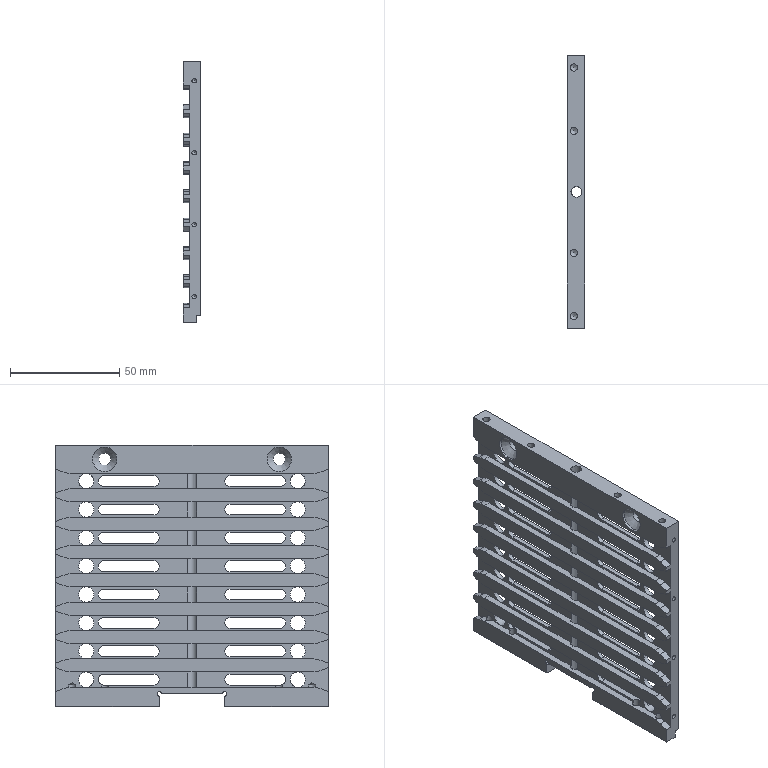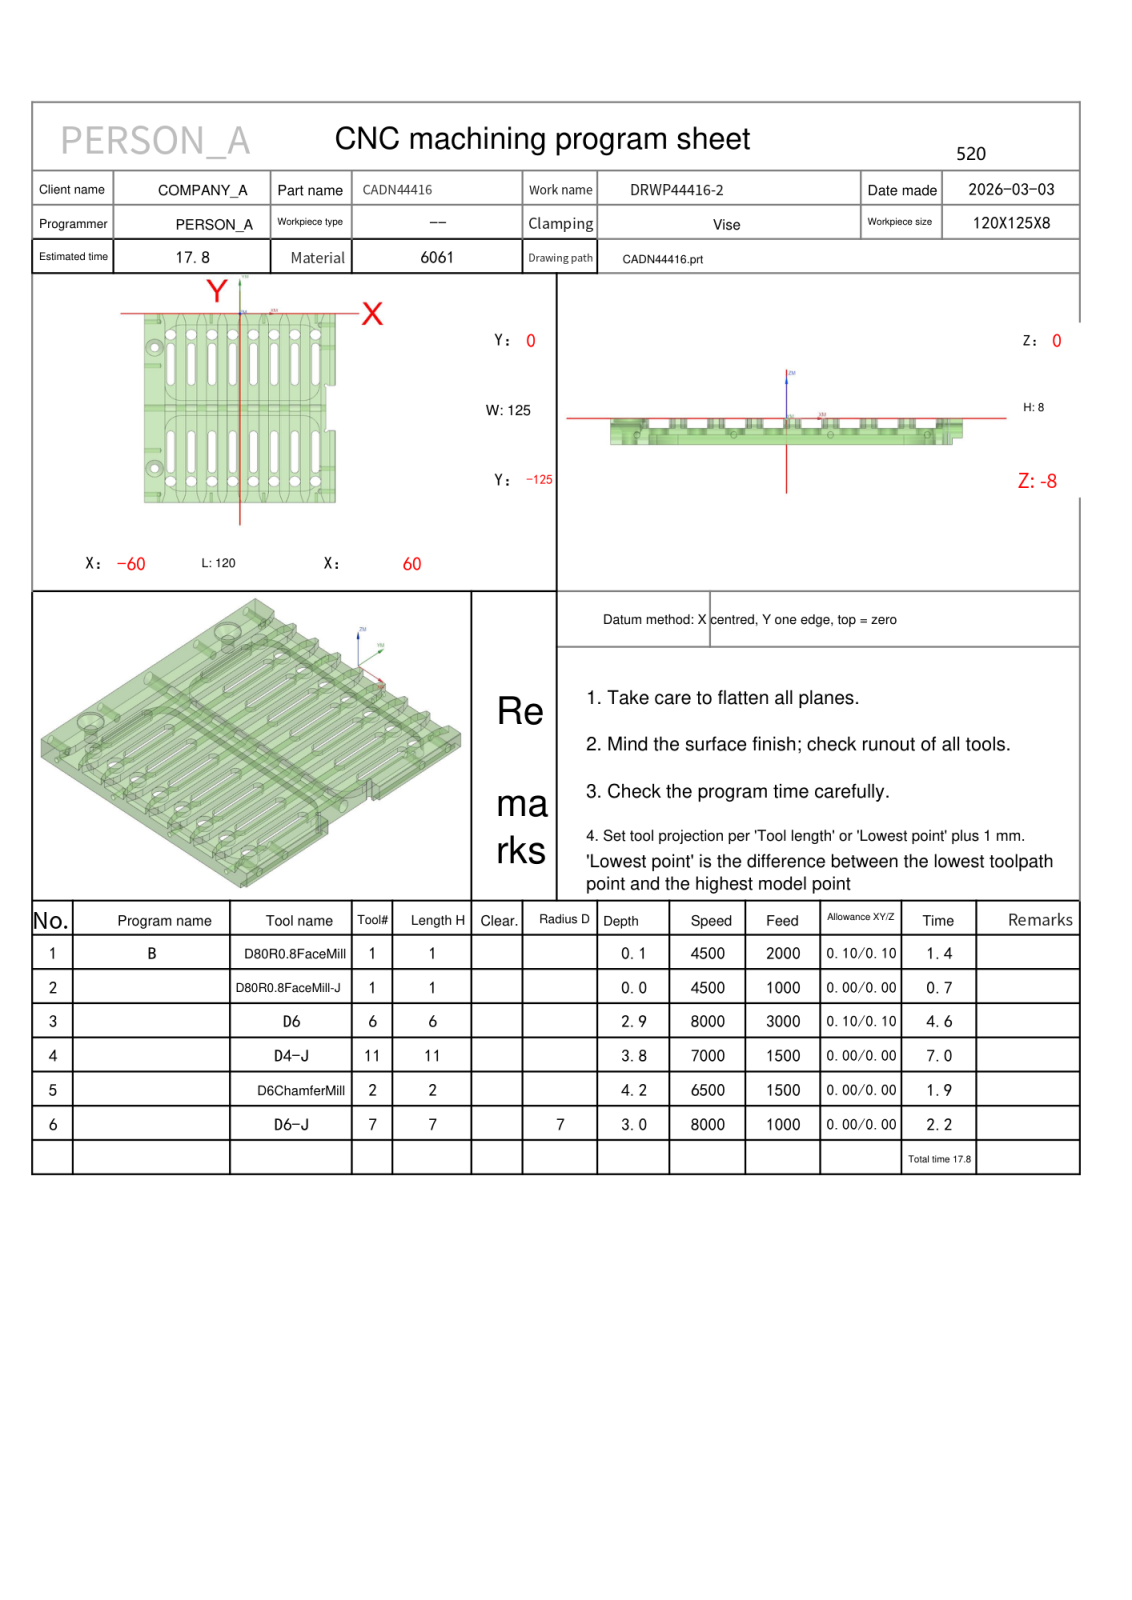NC program | NX | posted by the shop | part box 8 x 125 x 120 mm
Lines 1 to 1103 of 79132:
%
O0001
(Machine time: 19.00 MIN)
(===Total Tool:5===)
(T1=D80R0.8 FaceMill D=80.  R=0.8  D-  H01 Z=-0.   )
(T6=D6      D=6.   R=0.   D-  H06 Z=-2.9  )
(T11=D4-J   D=4.   R=0.   D-  H11 Z=-3.85 )
(T2=D6ChamferMill   D=6.   R=0.   D-  H02 Z=-4.2  )
(T7=D6-J    D=6.   R=0.   D7  H07 Z=-3.   )
G80 G90 G17 G49 G40
G91 G28 Z0
M01
N1 T01 M06
(D80R0.8 FaceMill  D=80. R=0.8 H=01 ce=0.10 di=0.10)
G00 G90 G54 X-112.097 Y-23.903 M03 S4500
G43 H01 Z50.
M08
Z3.525
G01 Z1.525 F2000.
X-100.097
X92.1
G02 X100.097 Y-31.9 I-.003 J-8.
G01 Y-37.403
Y-50.822
G02 X92.099 Y-58.82 I-8. J.002
G01 X-92.897
G03 X-100.097 Y-66.02 I0.0 J-7.2
G01 Y-85.737
G03 X-92.097 Y-93.737 I8. J0.0
G01 X100.097
X112.097
Z3.525
G00 X-112.097 Y-23.903
Z3.05
G01 Z1.05
X-100.097
X92.1
G02 X100.097 Y-31.9 I-.003 J-8.
G01 Y-37.403
Y-50.822
G02 X92.099 Y-58.82 I-8. J.002
G01 X-92.897
G03 X-100.097 Y-66.02 I0.0 J-7.2
G01 Y-85.737
G03 X-92.097 Y-93.737 I8. J0.0
G01 X100.097
X112.097
Z3.05
G00 X-112.097 Y-23.903
Z2.575
G01 Z.575
X-100.097
X92.1
G02 X100.097 Y-31.9 I-.003 J-8.
G01 Y-37.403
Y-50.822
G02 X92.099 Y-58.82 I-8. J.002
G01 X-92.897
G03 X-100.097 Y-66.02 I0.0 J-7.2
G01 Y-85.737
G03 X-92.097 Y-93.737 I8. J0.0
G01 X100.097
X112.097
Z2.575
G00 X-112.097 Y-23.903
Z2.1
G01 Z.1
X-100.097
X92.1
G02 X100.097 Y-31.9 I-.003 J-8.
G01 Y-37.403
Y-50.822
G02 X92.099 Y-58.82 I-8. J.002
G01 X-92.897
G03 X-100.097 Y-66.02 I0.0 J-7.2
G01 Y-85.737
G03 X-92.097 Y-93.737 I8. J0.0
G01 X100.097
X112.097
Z2.1
G00 Z50.
G91 G28 Z0.0
M05
M09
G91 G28 Z0.0
M01
N2 T01 M06
(D80R0.8 FaceMill-J  D=80. R=0.8 H=01 ce=0.00 di=0.00)
G00 G90 G54 X-111.999 Y-24.001 M03 S4500
G43 H01 Z50.
M08
Z2.
G01 Z0.0 F1000.
X-99.999
X92.002
G02 X99.999 Y-31.998 I-.003 J-8.
G01 Y-37.501
Y-50.823
G02 X92.002 Y-58.82 I-8. J.003
G01 X-92.799
G03 X-99.999 Y-66.02 I0.0 J-7.2
G01 Y-85.639
G03 X-91.999 Y-93.639 I8. J0.0
G01 X99.999
X111.999
Z2.
G00 Z50.
G91 G28 Z0.0
M05
M09
G91 G28 Z0.0
M01
N3 T06 M06
(D6  D=6. R=0. H=06 ce=0.10 di=0.10)
G00 G90 G54 X-43.5 Y-131. M03 S8000
G43 H06 Z11.805
M08
Z1.017
G01 Z-.483 F3000.
Y-127.94
X-46.773
X-44.69 Y-122.217
G03 X-43.9 Y-117.737 I-12.31 J4.48
G01 Y-7.263
G03 X-44.69 Y-2.783 I-13.1 J0.0
G01 X-46.773 Y2.94
X-40.227
X-42.31 Y-2.783
G03 X-43.1 Y-7.263 I12.31 J-4.48
G01 Y-117.737
G03 X-42.31 Y-122.217 I13.1 J0.0
G01 X-40.227 Y-127.94
X-43.5
X-44.
Y-131.
Z1.017
G00 X-43.5
Z.533
G01 Z-.967
Y-127.94
X-46.773
X-44.69 Y-122.217
G03 X-43.9 Y-117.737 I-12.31 J4.48
G01 Y-7.263
G03 X-44.69 Y-2.783 I-13.1 J0.0
G01 X-46.773 Y2.94
X-40.227
X-42.31 Y-2.783
G03 X-43.1 Y-7.263 I12.31 J-4.48
G01 Y-117.737
G03 X-42.31 Y-122.217 I13.1 J0.0
G01 X-40.227 Y-127.94
X-43.5
X-44.
Y-131.
Z.533
G00 X-43.5
Z.05
G01 Z-1.45
Y-127.94
X-46.773
X-44.69 Y-122.217
G03 X-43.9 Y-117.737 I-12.31 J4.48
G01 Y-7.263
G03 X-44.69 Y-2.783 I-13.1 J0.0
G01 X-46.773 Y2.94
X-40.227
X-42.31 Y-2.783
G03 X-43.1 Y-7.263 I12.31 J-4.48
G01 Y-117.737
G03 X-42.31 Y-122.217 I13.1 J0.0
G01 X-40.227 Y-127.94
X-43.5
X-44.
Y-131.
Z.05
G00 X-43.5
Z-.433
G01 Z-1.933
Y-127.94
X-46.773
X-44.69 Y-122.217
G03 X-43.9 Y-117.737 I-12.31 J4.48
G01 Y-7.263
G03 X-44.69 Y-2.783 I-13.1 J0.0
G01 X-46.773 Y2.94
X-40.227
X-42.31 Y-2.783
G03 X-43.1 Y-7.263 I12.31 J-4.48
G01 Y-117.737
G03 X-42.31 Y-122.217 I13.1 J0.0
G01 X-40.227 Y-127.94
X-43.5
X-44.
Y-131.
Z-.433
G00 X-43.5
Z-.917
G01 Z-2.417
Y-127.94
X-46.773
X-44.69 Y-122.217
G03 X-43.9 Y-117.737 I-12.31 J4.48
G01 Y-7.263
G03 X-44.69 Y-2.783 I-13.1 J0.0
G01 X-46.773 Y2.94
X-40.227
X-42.31 Y-2.783
G03 X-43.1 Y-7.263 I12.31 J-4.48
G01 Y-117.737
G03 X-42.31 Y-122.217 I13.1 J0.0
G01 X-40.227 Y-127.94
X-43.5
X-44.
Y-131.
Z-.917
G00 X-43.5
Z-1.4
G01 Z-2.9
Y-127.94
X-46.773
X-44.69 Y-122.217
G03 X-43.9 Y-117.737 I-12.31 J4.48
G01 Y-7.263
G03 X-44.69 Y-2.783 I-13.1 J0.0
G01 X-46.773 Y2.94
X-40.227
X-42.31 Y-2.783
G03 X-43.1 Y-7.263 I12.31 J-4.48
G01 Y-117.737
G03 X-42.31 Y-122.217 I13.1 J0.0
G01 X-40.227 Y-127.94
X-43.5
X-44.
Y-131.
Z-1.4
G00 Z3.
X-30.5
Z1.017
G01 Z-.483
Y-127.94
X-33.773
X-31.69 Y-122.217
G03 X-30.9 Y-117.737 I-12.31 J4.48
G01 Y-7.263
G03 X-31.69 Y-2.783 I-13.1 J0.0
G01 X-33.773 Y2.94
X-27.227
X-29.31 Y-2.783
G03 X-30.1 Y-7.263 I12.31 J-4.48
G01 Y-117.737
G03 X-29.31 Y-122.217 I13.1 J0.0
G01 X-27.227 Y-127.94
X-30.5
X-31.
Y-131.
Z1.017
G00 X-30.5
Z.533
G01 Z-.967
Y-127.94
X-33.773
X-31.69 Y-122.217
G03 X-30.9 Y-117.737 I-12.31 J4.48
G01 Y-7.263
G03 X-31.69 Y-2.783 I-13.1 J0.0
G01 X-33.773 Y2.94
X-27.227
X-29.31 Y-2.783
G03 X-30.1 Y-7.263 I12.31 J-4.48
G01 Y-117.737
G03 X-29.31 Y-122.217 I13.1 J0.0
G01 X-27.227 Y-127.94
X-30.5
X-31.
Y-131.
Z.533
G00 X-30.5
Z.05
G01 Z-1.45
Y-127.94
X-33.773
X-31.69 Y-122.217
G03 X-30.9 Y-117.737 I-12.31 J4.48
G01 Y-7.263
G03 X-31.69 Y-2.783 I-13.1 J0.0
G01 X-33.773 Y2.94
X-27.227
X-29.31 Y-2.783
G03 X-30.1 Y-7.263 I12.31 J-4.48
G01 Y-117.737
G03 X-29.31 Y-122.217 I13.1 J0.0
G01 X-27.227 Y-127.94
X-30.5
X-31.
Y-131.
Z.05
G00 X-30.5
Z-.433
G01 Z-1.933
Y-127.94
X-33.773
X-31.69 Y-122.217
G03 X-30.9 Y-117.737 I-12.31 J4.48
G01 Y-7.263
G03 X-31.69 Y-2.783 I-13.1 J0.0
G01 X-33.773 Y2.94
X-27.227
X-29.31 Y-2.783
G03 X-30.1 Y-7.263 I12.31 J-4.48
G01 Y-117.737
G03 X-29.31 Y-122.217 I13.1 J0.0
G01 X-27.227 Y-127.94
X-30.5
X-31.
Y-131.
Z-.433
G00 X-30.5
Z-.917
G01 Z-2.417
Y-127.94
X-33.773
X-31.69 Y-122.217
G03 X-30.9 Y-117.737 I-12.31 J4.48
G01 Y-7.263
G03 X-31.69 Y-2.783 I-13.1 J0.0
G01 X-33.773 Y2.94
X-27.227
X-29.31 Y-2.783
G03 X-30.1 Y-7.263 I12.31 J-4.48
G01 Y-117.737
G03 X-29.31 Y-122.217 I13.1 J0.0
G01 X-27.227 Y-127.94
X-30.5
X-31.
Y-131.
Z-.917
G00 X-30.5
Z-1.4
G01 Z-2.9
Y-127.94
X-33.773
X-31.69 Y-122.217
G03 X-30.9 Y-117.737 I-12.31 J4.48
G01 Y-7.263
G03 X-31.69 Y-2.783 I-13.1 J0.0
G01 X-33.773 Y2.94
X-27.227
X-29.31 Y-2.783
G03 X-30.1 Y-7.263 I12.31 J-4.48
G01 Y-117.737
G03 X-29.31 Y-122.217 I13.1 J0.0
G01 X-27.227 Y-127.94
X-30.5
X-31.
Y-131.
Z-1.4
G00 Z3.
X-17.5
Z1.017
G01 Z-.483
Y-127.94
X-20.773
X-18.69 Y-122.217
G03 X-17.9 Y-117.737 I-12.31 J4.48
G01 Y-7.263
G03 X-18.69 Y-2.783 I-13.1 J0.0
G01 X-20.773 Y2.94
X-14.227
X-16.31 Y-2.783
G03 X-17.1 Y-7.263 I12.31 J-4.48
G01 Y-117.737
G03 X-16.31 Y-122.217 I13.1 J0.0
G01 X-14.227 Y-127.94
X-17.5
X-18.
Y-131.
Z1.017
G00 X-17.5
Z.533
G01 Z-.967
Y-127.94
X-20.773
X-18.69 Y-122.217
G03 X-17.9 Y-117.737 I-12.31 J4.48
G01 Y-7.263
G03 X-18.69 Y-2.783 I-13.1 J0.0
G01 X-20.773 Y2.94
X-14.227
X-16.31 Y-2.783
G03 X-17.1 Y-7.263 I12.31 J-4.48
G01 Y-117.737
G03 X-16.31 Y-122.217 I13.1 J0.0
G01 X-14.227 Y-127.94
X-17.5
X-18.
Y-131.
Z.533
G00 X-17.5
Z.05
G01 Z-1.45
Y-127.94
X-20.773
X-18.69 Y-122.217
G03 X-17.9 Y-117.737 I-12.31 J4.48
G01 Y-7.263
G03 X-18.69 Y-2.783 I-13.1 J0.0
G01 X-20.773 Y2.94
X-14.227
X-16.31 Y-2.783
G03 X-17.1 Y-7.263 I12.31 J-4.48
G01 Y-117.737
G03 X-16.31 Y-122.217 I13.1 J0.0
G01 X-14.227 Y-127.94
X-17.5
X-18.
Y-131.
Z.05
G00 X-17.5
Z-.433
G01 Z-1.933
Y-127.94
X-20.773
X-18.69 Y-122.217
G03 X-17.9 Y-117.737 I-12.31 J4.48
G01 Y-7.263
G03 X-18.69 Y-2.783 I-13.1 J0.0
G01 X-20.773 Y2.94
X-14.227
X-16.31 Y-2.783
G03 X-17.1 Y-7.263 I12.31 J-4.48
G01 Y-117.737
G03 X-16.31 Y-122.217 I13.1 J0.0
G01 X-14.227 Y-127.94
X-17.5
X-18.
Y-131.
Z-.433
G00 X-17.5
Z-.917
G01 Z-2.417
Y-127.94
X-20.773
X-18.69 Y-122.217
G03 X-17.9 Y-117.737 I-12.31 J4.48
G01 Y-7.263
G03 X-18.69 Y-2.783 I-13.1 J0.0
G01 X-20.773 Y2.94
X-14.227
X-16.31 Y-2.783
G03 X-17.1 Y-7.263 I12.31 J-4.48
G01 Y-117.737
G03 X-16.31 Y-122.217 I13.1 J0.0
G01 X-14.227 Y-127.94
X-17.5
X-18.
Y-131.
Z-.917
G00 X-17.5
Z-1.4
G01 Z-2.9
Y-127.94
X-20.773
X-18.69 Y-122.217
G03 X-17.9 Y-117.737 I-12.31 J4.48
G01 Y-7.263
G03 X-18.69 Y-2.783 I-13.1 J0.0
G01 X-20.773 Y2.94
X-14.227
X-16.31 Y-2.783
G03 X-17.1 Y-7.263 I12.31 J-4.48
G01 Y-117.737
G03 X-16.31 Y-122.217 I13.1 J0.0
G01 X-14.227 Y-127.94
X-17.5
X-18.
Y-131.
Z-1.4
G00 Z3.
X-4.5
Z1.017
G01 Z-.483
Y-127.94
X-7.773
X-5.69 Y-122.217
G03 X-4.9 Y-117.737 I-12.31 J4.48
G01 Y-7.263
G03 X-5.69 Y-2.783 I-13.1 J0.0
G01 X-7.773 Y2.94
X-1.227
X-3.31 Y-2.783
G03 X-4.1 Y-7.263 I12.31 J-4.48
G01 Y-117.737
G03 X-3.31 Y-122.217 I13.1 J0.0
G01 X-1.227 Y-127.94
X-4.5
X-5.
Y-131.
Z1.017
G00 X-4.5
Z.533
G01 Z-.967
Y-127.94
X-7.773
X-5.69 Y-122.217
G03 X-4.9 Y-117.737 I-12.31 J4.48
G01 Y-7.263
G03 X-5.69 Y-2.783 I-13.1 J0.0
G01 X-7.773 Y2.94
X-1.227
X-3.31 Y-2.783
G03 X-4.1 Y-7.263 I12.31 J-4.48
G01 Y-117.737
G03 X-3.31 Y-122.217 I13.1 J0.0
G01 X-1.227 Y-127.94
X-4.5
X-5.
Y-131.
Z.533
G00 X-4.5
Z.05
G01 Z-1.45
Y-127.94
X-7.773
X-5.69 Y-122.217
G03 X-4.9 Y-117.737 I-12.31 J4.48
G01 Y-7.263
G03 X-5.69 Y-2.783 I-13.1 J0.0
G01 X-7.773 Y2.94
X-1.227
X-3.31 Y-2.783
G03 X-4.1 Y-7.263 I12.31 J-4.48
G01 Y-117.737
G03 X-3.31 Y-122.217 I13.1 J0.0
G01 X-1.227 Y-127.94
X-4.5
X-5.
Y-131.
Z.05
G00 X-4.5
Z-.433
G01 Z-1.933
Y-127.94
X-7.773
X-5.69 Y-122.217
G03 X-4.9 Y-117.737 I-12.31 J4.48
G01 Y-7.263
G03 X-5.69 Y-2.783 I-13.1 J0.0
G01 X-7.773 Y2.94
X-1.227
X-3.31 Y-2.783
G03 X-4.1 Y-7.263 I12.31 J-4.48
G01 Y-117.737
G03 X-3.31 Y-122.217 I13.1 J0.0
G01 X-1.227 Y-127.94
X-4.5
X-5.
Y-131.
Z-.433
G00 X-4.5
Z-.917
G01 Z-2.417
Y-127.94
X-7.773
X-5.69 Y-122.217
G03 X-4.9 Y-117.737 I-12.31 J4.48
G01 Y-7.263
G03 X-5.69 Y-2.783 I-13.1 J0.0
G01 X-7.773 Y2.94
X-1.227
X-3.31 Y-2.783
G03 X-4.1 Y-7.263 I12.31 J-4.48
G01 Y-117.737
G03 X-3.31 Y-122.217 I13.1 J0.0
G01 X-1.227 Y-127.94
X-4.5
X-5.
Y-131.
Z-.917
G00 X-4.5
Z-1.4
G01 Z-2.9
Y-127.94
X-7.773
X-5.69 Y-122.217
G03 X-4.9 Y-117.737 I-12.31 J4.48
G01 Y-7.263
G03 X-5.69 Y-2.783 I-13.1 J0.0
G01 X-7.773 Y2.94
X-1.227
X-3.31 Y-2.783
G03 X-4.1 Y-7.263 I12.31 J-4.48
G01 Y-117.737
G03 X-3.31 Y-122.217 I13.1 J0.0
G01 X-1.227 Y-127.94
X-4.5
X-5.
Y-131.
Z-1.4
G00 Z3.
X8.5
Z1.017
G01 Z-.483
Y-127.94
X5.227
X7.31 Y-122.217
G03 X8.1 Y-117.737 I-12.31 J4.48
G01 Y-7.263
G03 X7.31 Y-2.783 I-13.1 J0.0
G01 X5.227 Y2.94
X11.773
X9.69 Y-2.783
G03 X8.9 Y-7.263 I12.31 J-4.48
G01 Y-117.737
G03 X9.69 Y-122.217 I13.1 J0.0
G01 X11.773 Y-127.94
X8.5
X8.
Y-131.
Z1.017
G00 X8.5
Z.533
G01 Z-.967
Y-127.94
X5.227
X7.31 Y-122.217
G03 X8.1 Y-117.737 I-12.31 J4.48
G01 Y-7.263
G03 X7.31 Y-2.783 I-13.1 J0.0
G01 X5.227 Y2.94
X11.773
X9.69 Y-2.783
G03 X8.9 Y-7.263 I12.31 J-4.48
G01 Y-117.737
G03 X9.69 Y-122.217 I13.1 J0.0
G01 X11.773 Y-127.94
X8.5
X8.
Y-131.
Z.533
G00 X8.5
Z.05
G01 Z-1.45
Y-127.94
X5.227
X7.31 Y-122.217
G03 X8.1 Y-117.737 I-12.31 J4.48
G01 Y-7.263
G03 X7.31 Y-2.783 I-13.1 J0.0
G01 X5.227 Y2.94
X11.773
X9.69 Y-2.783
G03 X8.9 Y-7.263 I12.31 J-4.48
G01 Y-117.737
G03 X9.69 Y-122.217 I13.1 J0.0
G01 X11.773 Y-127.94
X8.5
X8.
Y-131.
Z.05
G00 X8.5
Z-.433
G01 Z-1.933
Y-127.94
X5.227
X7.31 Y-122.217
G03 X8.1 Y-117.737 I-12.31 J4.48
G01 Y-7.263
G03 X7.31 Y-2.783 I-13.1 J0.0
G01 X5.227 Y2.94
X11.773
X9.69 Y-2.783
G03 X8.9 Y-7.263 I12.31 J-4.48
G01 Y-117.737
G03 X9.69 Y-122.217 I13.1 J0.0
G01 X11.773 Y-127.94
X8.5
X8.
Y-131.
Z-.433
G00 X8.5
Z-.917
G01 Z-2.417
Y-127.94
X5.227
X7.31 Y-122.217
G03 X8.1 Y-117.737 I-12.31 J4.48
G01 Y-7.263
G03 X7.31 Y-2.783 I-13.1 J0.0
G01 X5.227 Y2.94
X11.773
X9.69 Y-2.783
G03 X8.9 Y-7.263 I12.31 J-4.48
G01 Y-117.737
G03 X9.69 Y-122.217 I13.1 J0.0
G01 X11.773 Y-127.94
X8.5
X8.
Y-131.
Z-.917
G00 X8.5
Z-1.4
G01 Z-2.9
Y-127.94
X5.227
X7.31 Y-122.217
G03 X8.1 Y-117.737 I-12.31 J4.48
G01 Y-7.263
G03 X7.31 Y-2.783 I-13.1 J0.0
G01 X5.227 Y2.94
X11.773
X9.69 Y-2.783
G03 X8.9 Y-7.263 I12.31 J-4.48
G01 Y-117.737
G03 X9.69 Y-122.217 I13.1 J0.0
G01 X11.773 Y-127.94
X8.5
X8.
Y-131.
Z-1.4
G00 Z3.
X21.427
Z1.017
G01 Z-.483
Y-127.94
X18.227
X20.31 Y-122.217
G03 X21.1 Y-117.737 I-12.31 J4.48
G01 Y-7.263
G03 X20.31 Y-2.783 I-13.1 J0.0
G01 X18.227 Y2.94
X18.336
X24.773
X22.69 Y-2.783
G03 X21.9 Y-7.263 I12.31 J-4.48
G01 Y-117.737
G03 X22.69 Y-122.217 I13.1 J0.0
G01 X24.773 Y-127.94
X24.627
X21.427
X20.927
Y-131.
Z1.017
G00 X21.427
Z.533
G01 Z-.967
Y-127.94
X18.227
X20.31 Y-122.217
G03 X21.1 Y-117.737 I-12.31 J4.48
G01 Y-7.263
G03 X20.31 Y-2.783 I-13.1 J0.0
G01 X18.227 Y2.94
X18.336
X24.773
X22.69 Y-2.783
G03 X21.9 Y-7.263 I12.31 J-4.48
G01 Y-117.737
G03 X22.69 Y-122.217 I13.1 J0.0
G01 X24.773 Y-127.94
X24.627
X21.427
X20.927
Y-131.
Z.533
G00 X21.427
Z.05
G01 Z-1.45
Y-127.94
X18.227
X20.31 Y-122.217
G03 X21.1 Y-117.737 I-12.31 J4.48
G01 Y-7.263
G03 X20.31 Y-2.783 I-13.1 J0.0
G01 X18.227 Y2.94
X18.336
X24.773
X22.69 Y-2.783
G03 X21.9 Y-7.263 I12.31 J-4.48
G01 Y-117.737
G03 X22.69 Y-122.217 I13.1 J0.0
G01 X24.773 Y-127.94
X24.627
X21.427
X20.927
Y-131.
Z.05
G00 X21.427
Z-.433
G01 Z-1.933
Y-127.94
X18.227
X20.31 Y-122.217
G03 X21.1 Y-117.737 I-12.31 J4.48
G01 Y-7.263
G03 X20.31 Y-2.783 I-13.1 J0.0
G01 X18.227 Y2.94
X18.336
X24.773
X22.69 Y-2.783
G03 X21.9 Y-7.263 I12.31 J-4.48
G01 Y-117.737
G03 X22.69 Y-122.217 I13.1 J0.0
G01 X24.773 Y-127.94
X24.627
X21.427
X20.927
Y-131.
Z-.433
G00 X21.427
Z-.917
G01 Z-2.417
Y-127.94
X18.227
X20.31 Y-122.217
G03 X21.1 Y-117.737 I-12.31 J4.48
G01 Y-7.263
G03 X20.31 Y-2.783 I-13.1 J0.0
G01 X18.227 Y2.94
X18.336
X24.773
X22.69 Y-2.783
G03 X21.9 Y-7.263 I12.31 J-4.48
G01 Y-117.737
G03 X22.69 Y-122.217 I13.1 J0.0
G01 X24.773 Y-127.94
X24.627
X21.427
X20.927
Y-131.
Z-.917
G00 X21.427
Z-1.4
G01 Z-2.9
Y-127.94
X18.227
X20.31 Y-122.217
G03 X21.1 Y-117.737 I-12.31 J4.48
G01 Y-7.263
G03 X20.31 Y-2.783 I-13.1 J0.0
G01 X18.227 Y2.94
X18.336
X24.773
X22.69 Y-2.783
G03 X21.9 Y-7.263 I12.31 J-4.48
G01 Y-117.737
G03 X22.69 Y-122.217 I13.1 J0.0
G01 X24.773 Y-127.94
X24.627
X21.427
X20.927
Y-131.
Z-1.4
G00 Z3.
X34.5
Z1.017
G01 Z-.483
Y-127.94
X31.227
X33.31 Y-122.217
G03 X34.1 Y-117.737 I-12.31 J4.48
G01 Y-7.263
G03 X33.31 Y-2.783 I-13.1 J0.0
G01 X31.227 Y2.94
X37.773
X35.69 Y-2.783
G03 X34.9 Y-7.263 I12.31 J-4.48
G01 Y-117.737
G03 X35.69 Y-122.217 I13.1 J0.0
G01 X37.773 Y-127.94
X34.5
X34.
Y-131.
Z1.017
G00 X34.5
Z.533
G01 Z-.967
Y-127.94
X31.227
X33.31 Y-122.217
G03 X34.1 Y-117.737 I-12.31 J4.48
G01 Y-7.263
G03 X33.31 Y-2.783 I-13.1 J0.0
G01 X31.227 Y2.94
X37.773
X35.69 Y-2.783
G03 X34.9 Y-7.263 I12.31 J-4.48
G01 Y-117.737
G03 X35.69 Y-122.217 I13.1 J0.0
G01 X37.773 Y-127.94
X34.5
X34.
Y-131.
Z.533
G00 X34.5
Z.05
G01 Z-1.45
Y-127.94
X31.227
X33.31 Y-122.217
G03 X34.1 Y-117.737 I-12.31 J4.48
G01 Y-7.263
G03 X33.31 Y-2.783 I-13.1 J0.0
G01 X31.227 Y2.94
X37.773
X35.69 Y-2.783
G03 X34.9 Y-7.263 I12.31 J-4.48
G01 Y-117.737
G03 X35.69 Y-122.217 I13.1 J0.0
G01 X37.773 Y-127.94
X34.5
X34.
Y-131.
Z.05
G00 X34.5
Z-.433
G01 Z-1.933
Y-127.94
X31.227
X33.31 Y-122.217
G03 X34.1 Y-117.737 I-12.31 J4.48
G01 Y-7.263
G03 X33.31 Y-2.783 I-13.1 J0.0
G01 X31.227 Y2.94
X37.773
X35.69 Y-2.783
G03 X34.9 Y-7.263 I12.31 J-4.48
G01 Y-117.737
G03 X35.69 Y-122.217 I13.1 J0.0
G01 X37.773 Y-127.94
X34.5
X34.
Y-131.
Z-.433
G00 X34.5
Z-.917
G01 Z-2.417
Y-127.94
X31.227
X33.31 Y-122.217
G03 X34.1 Y-117.737 I-12.31 J4.48
G01 Y-7.263
G03 X33.31 Y-2.783 I-13.1 J0.0
G01 X31.227 Y2.94
X37.773
X35.69 Y-2.783
G03 X34.9 Y-7.263 I12.31 J-4.48
G01 Y-117.737
G03 X35.69 Y-122.217 I13.1 J0.0
G01 X37.773 Y-127.94
X34.5
X34.
Y-131.
Z-.917
G00 X34.5
Z-1.4
G01 Z-2.9
Y-127.94
X31.227
X33.31 Y-122.217
G03 X34.1 Y-117.737 I-12.31 J4.48
G01 Y-7.263
G03 X33.31 Y-2.783 I-13.1 J0.0
G01 X31.227 Y2.94
X37.773
X35.69 Y-2.783
G03 X34.9 Y-7.263 I12.31 J-4.48
G01 Y-117.737
G03 X35.69 Y-122.217 I13.1 J0.0
G01 X37.773 Y-127.94
X34.5
X34.
Y-131.
Z-1.4
G00 Z3.
X47.5
Z1.017
G01 Z-.483
Y-127.94
X44.227
X46.31 Y-122.217
G03 X47.1 Y-117.737 I-12.31 J4.48
G01 Y-7.263
G03 X46.31 Y-2.783 I-13.1 J0.0
G01 X44.227 Y2.94
X50.773
X48.69 Y-2.783
G03 X47.9 Y-7.263 I12.31 J-4.48
G01 Y-117.737
G03 X48.69 Y-122.217 I13.1 J0.0
G01 X50.773 Y-127.94
X47.5
X47.
Y-131.
Z1.017
G00 X47.5
Z.533
G01 Z-.967
Y-127.94
X44.227
X46.31 Y-122.217
G03 X47.1 Y-117.737 I-12.31 J4.48
G01 Y-7.263
G03 X46.31 Y-2.783 I-13.1 J0.0
G01 X44.227 Y2.94
X50.773
X48.69 Y-2.783
G03 X47.9 Y-7.263 I12.31 J-4.48
G01 Y-117.737
G03 X48.69 Y-122.217 I13.1 J0.0
G01 X50.773 Y-127.94
X47.5
X47.
Y-131.
Z.533
G00 X47.5
Z.05
G01 Z-1.45
Y-127.94
X44.227
X46.31 Y-122.217
G03 X47.1 Y-117.737 I-12.31 J4.48
G01 Y-7.263
G03 X46.31 Y-2.783 I-13.1 J0.0
G01 X44.227 Y2.94
X50.773
X48.69 Y-2.783
G03 X47.9 Y-7.263 I12.31 J-4.48
G01 Y-117.737
G03 X48.69 Y-122.217 I13.1 J0.0
G01 X50.773 Y-127.94
X47.5
X47.
Y-131.
Z.05
G00 X47.5
Z-.433
G01 Z-1.933
Y-127.94
X44.227
X46.31 Y-122.217
G03 X47.1 Y-117.737 I-12.31 J4.48
G01 Y-7.263
G03 X46.31 Y-2.783 I-13.1 J0.0
G01 X44.227 Y2.94
X50.773
X48.69 Y-2.783
G03 X47.9 Y-7.263 I12.31 J-4.48
G01 Y-117.737
G03 X48.69 Y-122.217 I13.1 J0.0
G01 X50.773 Y-127.94
X47.5
X47.
Y-131.
Z-.433
G00 X47.5
Z-.917
G01 Z-2.417
Y-127.94
X44.227
X46.31 Y-122.217
G03 X47.1 Y-117.737 I-12.31 J4.48
G01 Y-7.263
G03 X46.31 Y-2.783 I-13.1 J0.0
G01 X44.227 Y2.94
X50.773
X48.69 Y-2.783
G03 X47.9 Y-7.263 I12.31 J-4.48
G01 Y-117.737
G03 X48.69 Y-122.217 I13.1 J0.0
G01 X50.773 Y-127.94
X47.5
X47.
Y-131.
Z-.917
G00 X47.5
Z-1.4
G01 Z-2.9
Y-127.94
X44.227
X46.31 Y-122.217
G03 X47.1 Y-117.737 I-12.31 J4.48
G01 Y-7.263
G03 X46.31 Y-2.783 I-13.1 J0.0
G01 X44.227 Y2.94
X50.773
X48.69 Y-2.783
G03 X47.9 Y-7.263 I12.31 J-4.48
G01 Y-117.737
G03 X48.69 Y-122.217 I13.1 J0.0
G01 X50.773 Y-127.94
X47.5
X47.
Y-131.
Z-1.4
G00 Z11.805
G91 G28 Z0.0
M05
M09
G91 G28 Z0.0
M01